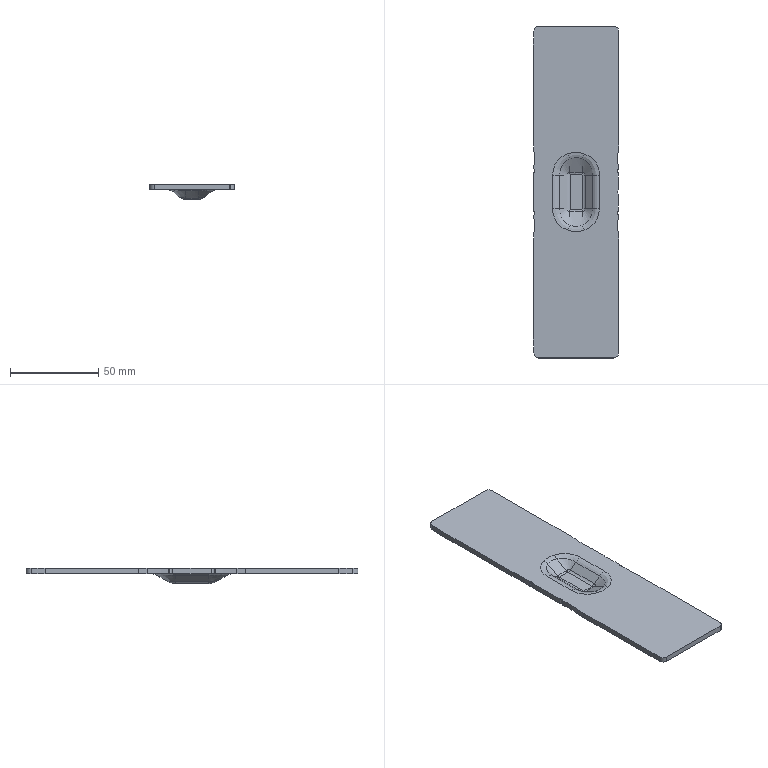Part | STEP file | 1_id366_x_t | 1 solid | 87 faces | box 48.382 x 188.49 x 8.554 mm | volume 28332 mm3 | spline 36 | cylinder 27 | plane 20 | other 4 | commonest cylinder face diameters 3 x8 6 x8 12.15 x4 101.133 x4 2205 x2 9.576 x1